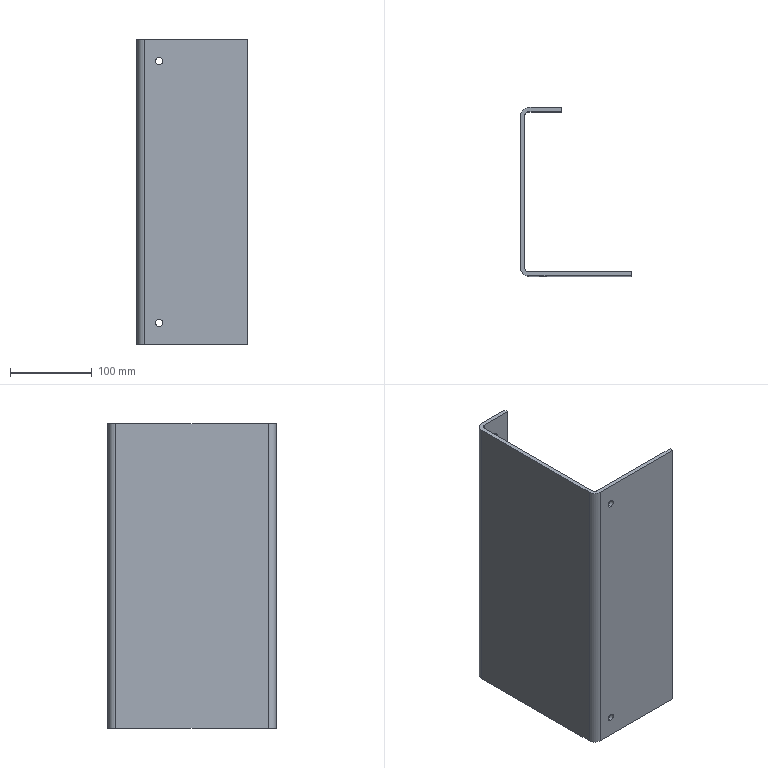Part | SolidWorks | features ExtruThin 1, ICE 1, LPattern 1 | 1 solid | 22 faces | box 135 x 206 x 372 mm | volume 695413 mm3 | cylinder 12 | plane 10 | commonest cylinder face diameters 9 x8 10 x2 20 x2
STEP:
#1=CARTESIAN_POINT('',(27.5,201.,21.5));
#2=VERTEX_POINT('',#1);
#3=CARTESIAN_POINT('',(27.5,201.,30.5));
#4=VERTEX_POINT('',#3);
#5=CARTESIAN_POINT('',(27.5,201.,26.));
#6=DIRECTION('',(0.,1.,0.));
#7=DIRECTION('',(0.,0.,1.));
#8=AXIS2_PLACEMENT_3D('',#5,#6,#7);
#9=CIRCLE('',#8,4.5);
#10=EDGE_CURVE('',#2,#4,#9,.T.);
#11=ORIENTED_EDGE('',*,*,#10,.F.);
#12=CARTESIAN_POINT('',(27.5,206.,21.5));
#13=VERTEX_POINT('',#12);
#14=CARTESIAN_POINT('',(27.5,0.,21.5));
#15=DIRECTION('',(0.,1.,0.));
#16=VECTOR('',#15,1000.);
#17=LINE('',#14,#16);
#18=EDGE_CURVE('',#2,#13,#17,.T.);
#19=ORIENTED_EDGE('',*,*,#18,.T.);
#20=CARTESIAN_POINT('',(27.5,206.,30.5));
#21=VERTEX_POINT('',#20);
#22=CARTESIAN_POINT('',(27.5,206.,26.));
#23=DIRECTION('',(0.,1.,0.));
#24=DIRECTION('',(0.,0.,1.));
#25=AXIS2_PLACEMENT_3D('',#22,#23,#24);
#26=CIRCLE('',#25,4.5);
#27=EDGE_CURVE('',#13,#21,#26,.T.);
#28=ORIENTED_EDGE('',*,*,#27,.T.);
#29=CARTESIAN_POINT('',(27.5,0.,30.5));
#30=DIRECTION('',(0.,1.,0.));
#31=VECTOR('',#30,1000.);
#32=LINE('',#29,#31);
#33=EDGE_CURVE('',#4,#21,#32,.T.);
#34=ORIENTED_EDGE('',*,*,#33,.F.);
#35=EDGE_LOOP('',(#11,#19,#28,#34));
#36=FACE_OUTER_BOUND('',#35,.T.);
#37=CARTESIAN_POINT('',(27.5,0.,26.));
#38=DIRECTION('',(0.,1.,0.));
#39=DIRECTION('',(0.,0.,1.));
#40=AXIS2_PLACEMENT_3D('',#37,#38,#39);
#41=CYLINDRICAL_SURFACE('',#40,4.5);
#42=ADVANCED_FACE('',(#36),#41,.F.);
#43=CARTESIAN_POINT('',(27.5,0.,21.5));
#44=VERTEX_POINT('',#43);
#45=CARTESIAN_POINT('',(27.5,0.,30.5));
#46=VERTEX_POINT('',#45);
#47=CARTESIAN_POINT('',(27.5,0.,26.));
#48=DIRECTION('',(0.,1.,0.));
#49=DIRECTION('',(0.,0.,1.));
#50=AXIS2_PLACEMENT_3D('',#47,#48,#49);
#51=CIRCLE('',#50,4.5);
#52=EDGE_CURVE('',#44,#46,#51,.T.);
#53=ORIENTED_EDGE('',*,*,#52,.F.);
#54=CARTESIAN_POINT('',(27.5,5.,21.5));
#55=VERTEX_POINT('',#54);
#56=CARTESIAN_POINT('',(27.5,0.,21.5));
#57=DIRECTION('',(0.,1.,0.));
#58=VECTOR('',#57,1000.);
#59=LINE('',#56,#58);
#60=EDGE_CURVE('',#44,#55,#59,.T.);
#61=ORIENTED_EDGE('',*,*,#60,.T.);
#62=CARTESIAN_POINT('',(27.5,5.,30.5));
#63=VERTEX_POINT('',#62);
#64=CARTESIAN_POINT('',(27.5,5.,26.));
#65=DIRECTION('',(0.,-1.,0.));
#66=DIRECTION('',(0.,0.,-1.));
#67=AXIS2_PLACEMENT_3D('',#64,#65,#66);
#68=CIRCLE('',#67,4.5);
#69=EDGE_CURVE('',#63,#55,#68,.T.);
#70=ORIENTED_EDGE('',*,*,#69,.F.);
#71=CARTESIAN_POINT('',(27.5,0.,30.5));
#72=DIRECTION('',(0.,1.,0.));
#73=VECTOR('',#72,1000.);
#74=LINE('',#71,#73);
#75=EDGE_CURVE('',#46,#63,#74,.T.);
#76=ORIENTED_EDGE('',*,*,#75,.F.);
#77=EDGE_LOOP('',(#53,#61,#70,#76));
#78=FACE_OUTER_BOUND('',#77,.T.);
#79=CARTESIAN_POINT('',(27.5,0.,26.));
#80=DIRECTION('',(0.,1.,0.));
#81=DIRECTION('',(0.,0.,1.));
#82=AXIS2_PLACEMENT_3D('',#79,#80,#81);
#83=CYLINDRICAL_SURFACE('',#82,4.5);
#84=ADVANCED_FACE('',(#78),#83,.F.);
#85=CARTESIAN_POINT('',(27.5,201.,341.5));
#86=VERTEX_POINT('',#85);
#87=CARTESIAN_POINT('',(27.5,201.,350.5));
#88=VERTEX_POINT('',#87);
#89=CARTESIAN_POINT('',(27.5,201.,346.));
#90=DIRECTION('',(0.,1.,0.));
#91=DIRECTION('',(0.,0.,1.));
#92=AXIS2_PLACEMENT_3D('',#89,#90,#91);
#93=CIRCLE('',#92,4.5);
#94=EDGE_CURVE('',#86,#88,#93,.T.);
#95=ORIENTED_EDGE('',*,*,#94,.F.);
#96=CARTESIAN_POINT('',(27.5,206.,341.5));
#97=VERTEX_POINT('',#96);
#98=CARTESIAN_POINT('',(27.5,0.,341.5));
#99=DIRECTION('',(0.,1.,0.));
#100=VECTOR('',#99,1000.);
#101=LINE('',#98,#100);
#102=EDGE_CURVE('',#86,#97,#101,.T.);
#103=ORIENTED_EDGE('',*,*,#102,.T.);
#104=CARTESIAN_POINT('',(27.5,206.,350.5));
#105=VERTEX_POINT('',#104);
#106=CARTESIAN_POINT('',(27.5,206.,346.));
#107=DIRECTION('',(0.,1.,0.));
#108=DIRECTION('',(0.,0.,1.));
#109=AXIS2_PLACEMENT_3D('',#106,#107,#108);
#110=CIRCLE('',#109,4.5);
#111=EDGE_CURVE('',#97,#105,#110,.T.);
#112=ORIENTED_EDGE('',*,*,#111,.T.);
#113=CARTESIAN_POINT('',(27.5,0.,350.5));
#114=DIRECTION('',(0.,1.,0.));
#115=VECTOR('',#114,1000.);
#116=LINE('',#113,#115);
#117=EDGE_CURVE('',#88,#105,#116,.T.);
#118=ORIENTED_EDGE('',*,*,#117,.F.);
#119=EDGE_LOOP('',(#95,#103,#112,#118));
#120=FACE_OUTER_BOUND('',#119,.T.);
#121=CARTESIAN_POINT('',(27.5,0.,346.));
#122=DIRECTION('',(0.,1.,0.));
#123=DIRECTION('',(0.,0.,1.));
#124=AXIS2_PLACEMENT_3D('',#121,#122,#123);
#125=CYLINDRICAL_SURFACE('',#124,4.5);
#126=ADVANCED_FACE('',(#120),#125,.F.);
#127=CARTESIAN_POINT('',(27.5,0.,341.5));
#128=VERTEX_POINT('',#127);
#129=CARTESIAN_POINT('',(27.5,0.,350.5));
#130=VERTEX_POINT('',#129);
#131=CARTESIAN_POINT('',(27.5,0.,346.));
#132=DIRECTION('',(0.,1.,0.));
#133=DIRECTION('',(0.,0.,1.));
#134=AXIS2_PLACEMENT_3D('',#131,#132,#133);
#135=CIRCLE('',#134,4.5);
#136=EDGE_CURVE('',#128,#130,#135,.T.);
#137=ORIENTED_EDGE('',*,*,#136,.F.);
#138=CARTESIAN_POINT('',(27.5,5.,341.5));
#139=VERTEX_POINT('',#138);
#140=CARTESIAN_POINT('',(27.5,0.,341.5));
#141=DIRECTION('',(0.,1.,0.));
#142=VECTOR('',#141,1000.);
#143=LINE('',#140,#142);
#144=EDGE_CURVE('',#128,#139,#143,.T.);
#145=ORIENTED_EDGE('',*,*,#144,.T.);
#146=CARTESIAN_POINT('',(27.5,5.,350.5));
#147=VERTEX_POINT('',#146);
#148=CARTESIAN_POINT('',(27.5,5.,346.));
#149=DIRECTION('',(0.,-1.,0.));
#150=DIRECTION('',(0.,0.,-1.));
#151=AXIS2_PLACEMENT_3D('',#148,#149,#150);
#152=CIRCLE('',#151,4.5);
#153=EDGE_CURVE('',#147,#139,#152,.T.);
#154=ORIENTED_EDGE('',*,*,#153,.F.);
#155=CARTESIAN_POINT('',(27.5,0.,350.5));
#156=DIRECTION('',(0.,1.,0.));
#157=VECTOR('',#156,1000.);
#158=LINE('',#155,#157);
#159=EDGE_CURVE('',#130,#147,#158,.T.);
#160=ORIENTED_EDGE('',*,*,#159,.F.);
#161=EDGE_LOOP('',(#137,#145,#154,#160));
#162=FACE_OUTER_BOUND('',#161,.T.);
#163=CARTESIAN_POINT('',(27.5,0.,346.));
#164=DIRECTION('',(0.,1.,0.));
#165=DIRECTION('',(0.,0.,1.));
#166=AXIS2_PLACEMENT_3D('',#163,#164,#165);
#167=CYLINDRICAL_SURFACE('',#166,4.5);
#168=ADVANCED_FACE('',(#162),#167,.F.);
#169=CARTESIAN_POINT('',(27.5,201.,26.));
#170=DIRECTION('',(0.,1.,0.));
#171=DIRECTION('',(0.,0.,1.));
#172=AXIS2_PLACEMENT_3D('',#169,#170,#171);
#173=CIRCLE('',#172,4.5);
#174=EDGE_CURVE('',#4,#2,#173,.T.);
#175=ORIENTED_EDGE('',*,*,#174,.T.);
#176=ORIENTED_EDGE('',*,*,#10,.T.);
#177=EDGE_LOOP('',(#175,#176));
#178=FACE_BOUND('',#177,.T.);
#179=CARTESIAN_POINT('',(27.5,201.,346.));
#180=DIRECTION('',(0.,1.,0.));
#181=DIRECTION('',(0.,0.,1.));
#182=AXIS2_PLACEMENT_3D('',#179,#180,#181);
#183=CIRCLE('',#182,4.5);
#184=EDGE_CURVE('',#88,#86,#183,.T.);
#185=ORIENTED_EDGE('',*,*,#184,.T.);
#186=ORIENTED_EDGE('',*,*,#94,.T.);
#187=EDGE_LOOP('',(#185,#186));
#188=FACE_BOUND('',#187,.T.);
#189=CARTESIAN_POINT('',(10.,201.,0.));
#190=VERTEX_POINT('',#189);
#191=CARTESIAN_POINT('',(50.,201.,0.));
#192=VERTEX_POINT('',#191);
#193=CARTESIAN_POINT('',(10.,201.,0.));
#194=DIRECTION('',(1.,0.,0.));
#195=VECTOR('',#194,1000.);
#196=LINE('',#193,#195);
#197=EDGE_CURVE('',#190,#192,#196,.T.);
#198=ORIENTED_EDGE('',*,*,#197,.T.);
#199=CARTESIAN_POINT('',(50.,201.,372.));
#200=VERTEX_POINT('',#199);
#201=CARTESIAN_POINT('',(50.,201.,372.));
#202=DIRECTION('',(0.,0.,-1.));
#203=VECTOR('',#202,1000.);
#204=LINE('',#201,#203);
#205=EDGE_CURVE('',#200,#192,#204,.T.);
#206=ORIENTED_EDGE('',*,*,#205,.F.);
#207=CARTESIAN_POINT('',(10.,201.,372.));
#208=VERTEX_POINT('',#207);
#209=CARTESIAN_POINT('',(10.,201.,372.));
#210=DIRECTION('',(1.,0.,0.));
#211=VECTOR('',#210,1000.);
#212=LINE('',#209,#211);
#213=EDGE_CURVE('',#208,#200,#212,.T.);
#214=ORIENTED_EDGE('',*,*,#213,.F.);
#215=CARTESIAN_POINT('',(10.,201.,372.));
#216=DIRECTION('',(0.,0.,-1.));
#217=VECTOR('',#216,1000.);
#218=LINE('',#215,#217);
#219=EDGE_CURVE('',#208,#190,#218,.T.);
#220=ORIENTED_EDGE('',*,*,#219,.T.);
#221=EDGE_LOOP('',(#198,#206,#214,#220));
#222=FACE_OUTER_BOUND('',#221,.T.);
#223=CARTESIAN_POINT('',(10.,201.,372.));
#224=DIRECTION('',(0.,1.,0.));
#225=DIRECTION('',(0.,0.,1.));
#226=AXIS2_PLACEMENT_3D('',#223,#224,#225);
#227=PLANE('',#226);
#228=ADVANCED_FACE('',(#178,#188,#222),#227,.F.);
#229=CARTESIAN_POINT('',(50.,206.,0.));
#230=VERTEX_POINT('',#229);
#231=CARTESIAN_POINT('',(50.,206.,0.));
#232=DIRECTION('',(0.,-1.,0.));
#233=VECTOR('',#232,1000.);
#234=LINE('',#231,#233);
#235=EDGE_CURVE('',#230,#192,#234,.T.);
#236=ORIENTED_EDGE('',*,*,#235,.F.);
#237=CARTESIAN_POINT('',(50.,206.,372.));
#238=VERTEX_POINT('',#237);
#239=CARTESIAN_POINT('',(50.,206.,372.));
#240=DIRECTION('',(0.,0.,-1.));
#241=VECTOR('',#240,1000.);
#242=LINE('',#239,#241);
#243=EDGE_CURVE('',#238,#230,#242,.T.);
#244=ORIENTED_EDGE('',*,*,#243,.F.);
#245=CARTESIAN_POINT('',(50.,206.,372.));
#246=DIRECTION('',(0.,-1.,0.));
#247=VECTOR('',#246,1000.);
#248=LINE('',#245,#247);
#249=EDGE_CURVE('',#238,#200,#248,.T.);
#250=ORIENTED_EDGE('',*,*,#249,.T.);
#251=ORIENTED_EDGE('',*,*,#205,.T.);
#252=EDGE_LOOP('',(#236,#244,#250,#251));
#253=FACE_OUTER_BOUND('',#252,.T.);
#254=CARTESIAN_POINT('',(50.,206.,372.));
#255=DIRECTION('',(1.,0.,0.));
#256=DIRECTION('',(0.,0.,-1.));
#257=AXIS2_PLACEMENT_3D('',#254,#255,#256);
#258=PLANE('',#257);
#259=ADVANCED_FACE('',(#253),#258,.T.);
#260=CARTESIAN_POINT('',(27.5,206.,26.));
#261=DIRECTION('',(0.,1.,0.));
#262=DIRECTION('',(0.,0.,1.));
#263=AXIS2_PLACEMENT_3D('',#260,#261,#262);
#264=CIRCLE('',#263,4.5);
#265=EDGE_CURVE('',#21,#13,#264,.T.);
#266=ORIENTED_EDGE('',*,*,#265,.F.);
#267=ORIENTED_EDGE('',*,*,#27,.F.);
#268=EDGE_LOOP('',(#266,#267));
#269=FACE_BOUND('',#268,.T.);
#270=CARTESIAN_POINT('',(27.5,206.,346.));
#271=DIRECTION('',(0.,1.,0.));
#272=DIRECTION('',(0.,0.,1.));
#273=AXIS2_PLACEMENT_3D('',#270,#271,#272);
#274=CIRCLE('',#273,4.5);
#275=EDGE_CURVE('',#105,#97,#274,.T.);
#276=ORIENTED_EDGE('',*,*,#275,.F.);
#277=ORIENTED_EDGE('',*,*,#111,.F.);
#278=EDGE_LOOP('',(#276,#277));
#279=FACE_BOUND('',#278,.T.);
#280=CARTESIAN_POINT('',(10.,206.,0.));
#281=VERTEX_POINT('',#280);
#282=CARTESIAN_POINT('',(10.,206.,0.));
#283=DIRECTION('',(1.,0.,0.));
#284=VECTOR('',#283,1000.);
#285=LINE('',#282,#284);
#286=EDGE_CURVE('',#281,#230,#285,.T.);
#287=ORIENTED_EDGE('',*,*,#286,.F.);
#288=CARTESIAN_POINT('',(10.,206.,372.));
#289=VERTEX_POINT('',#288);
#290=CARTESIAN_POINT('',(10.,206.,372.));
#291=DIRECTION('',(0.,0.,-1.));
#292=VECTOR('',#291,1000.);
#293=LINE('',#290,#292);
#294=EDGE_CURVE('',#289,#281,#293,.T.);
#295=ORIENTED_EDGE('',*,*,#294,.F.);
#296=CARTESIAN_POINT('',(10.,206.,372.));
#297=DIRECTION('',(1.,0.,0.));
#298=VECTOR('',#297,1000.);
#299=LINE('',#296,#298);
#300=EDGE_CURVE('',#289,#238,#299,.T.);
#301=ORIENTED_EDGE('',*,*,#300,.T.);
#302=ORIENTED_EDGE('',*,*,#243,.T.);
#303=EDGE_LOOP('',(#287,#295,#301,#302));
#304=FACE_OUTER_BOUND('',#303,.T.);
#305=CARTESIAN_POINT('',(10.,206.,372.));
#306=DIRECTION('',(0.,1.,0.));
#307=DIRECTION('',(0.,0.,1.));
#308=AXIS2_PLACEMENT_3D('',#305,#306,#307);
#309=PLANE('',#308);
#310=ADVANCED_FACE('',(#269,#279,#304),#309,.T.);
#311=CARTESIAN_POINT('',(0.,196.,0.));
#312=VERTEX_POINT('',#311);
#313=CARTESIAN_POINT('',(10.,196.,0.));
#314=DIRECTION('',(0.,0.,-1.));
#315=DIRECTION('',(1.,0.,0.));
#316=AXIS2_PLACEMENT_3D('',#313,#314,#315);
#317=CIRCLE('',#316,10.);
#318=EDGE_CURVE('',#312,#281,#317,.T.);
#319=ORIENTED_EDGE('',*,*,#318,.F.);
#320=CARTESIAN_POINT('',(0.,196.,372.));
#321=VERTEX_POINT('',#320);
#322=CARTESIAN_POINT('',(0.,196.,372.));
#323=DIRECTION('',(0.,0.,-1.));
#324=VECTOR('',#323,1000.);
#325=LINE('',#322,#324);
#326=EDGE_CURVE('',#321,#312,#325,.T.);
#327=ORIENTED_EDGE('',*,*,#326,.F.);
#328=CARTESIAN_POINT('',(10.,196.,372.));
#329=DIRECTION('',(0.,0.,-1.));
#330=DIRECTION('',(1.,0.,0.));
#331=AXIS2_PLACEMENT_3D('',#328,#329,#330);
#332=CIRCLE('',#331,10.);
#333=EDGE_CURVE('',#321,#289,#332,.T.);
#334=ORIENTED_EDGE('',*,*,#333,.T.);
#335=ORIENTED_EDGE('',*,*,#294,.T.);
#336=EDGE_LOOP('',(#319,#327,#334,#335));
#337=FACE_OUTER_BOUND('',#336,.T.);
#338=CARTESIAN_POINT('',(10.,196.,372.));
#339=DIRECTION('',(0.,0.,-1.));
#340=DIRECTION('',(-1.,0.,0.));
#341=AXIS2_PLACEMENT_3D('',#338,#339,#340);
#342=CYLINDRICAL_SURFACE('',#341,10.);
#343=ADVANCED_FACE('',(#337),#342,.T.);
#344=CARTESIAN_POINT('',(0.,10.,0.));
#345=VERTEX_POINT('',#344);
#346=CARTESIAN_POINT('',(0.,10.,0.));
#347=DIRECTION('',(0.,1.,0.));
#348=VECTOR('',#347,1000.);
#349=LINE('',#346,#348);
#350=EDGE_CURVE('',#345,#312,#349,.T.);
#351=ORIENTED_EDGE('',*,*,#350,.F.);
#352=CARTESIAN_POINT('',(0.,10.,372.));
#353=VERTEX_POINT('',#352);
#354=CARTESIAN_POINT('',(0.,10.,372.));
#355=DIRECTION('',(0.,0.,-1.));
#356=VECTOR('',#355,1000.);
#357=LINE('',#354,#356);
#358=EDGE_CURVE('',#353,#345,#357,.T.);
#359=ORIENTED_EDGE('',*,*,#358,.F.);
#360=CARTESIAN_POINT('',(0.,10.,372.));
#361=DIRECTION('',(0.,1.,0.));
#362=VECTOR('',#361,1000.);
#363=LINE('',#360,#362);
#364=EDGE_CURVE('',#353,#321,#363,.T.);
#365=ORIENTED_EDGE('',*,*,#364,.T.);
#366=ORIENTED_EDGE('',*,*,#326,.T.);
#367=EDGE_LOOP('',(#351,#359,#365,#366));
#368=FACE_OUTER_BOUND('',#367,.T.);
#369=CARTESIAN_POINT('',(0.,10.,372.));
#370=DIRECTION('',(-1.,0.,0.));
#371=DIRECTION('',(0.,0.,1.));
#372=AXIS2_PLACEMENT_3D('',#369,#370,#371);
#373=PLANE('',#372);
#374=ADVANCED_FACE('',(#368),#373,.T.);
#375=CARTESIAN_POINT('',(10.,0.,0.));
#376=VERTEX_POINT('',#375);
#377=CARTESIAN_POINT('',(10.,10.,0.));
#378=DIRECTION('',(0.,0.,-1.));
#379=DIRECTION('',(-1.,0.,0.));
#380=AXIS2_PLACEMENT_3D('',#377,#378,#379);
#381=CIRCLE('',#380,10.);
#382=EDGE_CURVE('',#376,#345,#381,.T.);
#383=ORIENTED_EDGE('',*,*,#382,.F.);
#384=CARTESIAN_POINT('',(10.,0.,372.));
#385=VERTEX_POINT('',#384);
#386=CARTESIAN_POINT('',(10.,0.,372.));
#387=DIRECTION('',(0.,0.,-1.));
#388=VECTOR('',#387,1000.);
#389=LINE('',#386,#388);
#390=EDGE_CURVE('',#385,#376,#389,.T.);
#391=ORIENTED_EDGE('',*,*,#390,.F.);
#392=CARTESIAN_POINT('',(10.,10.,372.));
#393=DIRECTION('',(0.,0.,-1.));
#394=DIRECTION('',(-1.,0.,0.));
#395=AXIS2_PLACEMENT_3D('',#392,#393,#394);
#396=CIRCLE('',#395,10.);
#397=EDGE_CURVE('',#385,#353,#396,.T.);
#398=ORIENTED_EDGE('',*,*,#397,.T.);
#399=ORIENTED_EDGE('',*,*,#358,.T.);
#400=EDGE_LOOP('',(#383,#391,#398,#399));
#401=FACE_OUTER_BOUND('',#400,.T.);
#402=CARTESIAN_POINT('',(10.,10.,372.));
#403=DIRECTION('',(0.,0.,-1.));
#404=DIRECTION('',(-1.,0.,0.));
#405=AXIS2_PLACEMENT_3D('',#402,#403,#404);
#406=CYLINDRICAL_SURFACE('',#405,10.);
#407=ADVANCED_FACE('',(#401),#406,.T.);
#408=CARTESIAN_POINT('',(27.5,0.,26.));
#409=DIRECTION('',(0.,1.,0.));
#410=DIRECTION('',(0.,0.,1.));
#411=AXIS2_PLACEMENT_3D('',#408,#409,#410);
#412=CIRCLE('',#411,4.5);
#413=EDGE_CURVE('',#46,#44,#412,.T.);
#414=ORIENTED_EDGE('',*,*,#413,.T.);
#415=ORIENTED_EDGE('',*,*,#52,.T.);
#416=EDGE_LOOP('',(#414,#415));
#417=FACE_BOUND('',#416,.T.);
#418=CARTESIAN_POINT('',(27.5,0.,346.));
#419=DIRECTION('',(0.,1.,0.));
#420=DIRECTION('',(0.,0.,1.));
#421=AXIS2_PLACEMENT_3D('',#418,#419,#420);
#422=CIRCLE('',#421,4.5);
#423=EDGE_CURVE('',#130,#128,#422,.T.);
#424=ORIENTED_EDGE('',*,*,#423,.T.);
#425=ORIENTED_EDGE('',*,*,#136,.T.);
#426=EDGE_LOOP('',(#424,#425));
#427=FACE_BOUND('',#426,.T.);
#428=CARTESIAN_POINT('',(135.,0.,0.));
#429=VERTEX_POINT('',#428);
#430=CARTESIAN_POINT('',(10.,0.,0.));
#431=DIRECTION('',(-1.,0.,0.));
#432=VECTOR('',#431,1000.);
#433=LINE('',#430,#432);
#434=EDGE_CURVE('',#429,#376,#433,.T.);
#435=ORIENTED_EDGE('',*,*,#434,.F.);
#436=CARTESIAN_POINT('',(135.,0.,372.));
#437=VERTEX_POINT('',#436);
#438=CARTESIAN_POINT('',(135.,0.,372.));
#439=DIRECTION('',(0.,0.,-1.));
#440=VECTOR('',#439,1000.);
#441=LINE('',#438,#440);
#442=EDGE_CURVE('',#437,#429,#441,.T.);
#443=ORIENTED_EDGE('',*,*,#442,.F.);
#444=CARTESIAN_POINT('',(10.,0.,372.));
#445=DIRECTION('',(-1.,0.,0.));
#446=VECTOR('',#445,1000.);
#447=LINE('',#444,#446);
#448=EDGE_CURVE('',#437,#385,#447,.T.);
#449=ORIENTED_EDGE('',*,*,#448,.T.);
#450=ORIENTED_EDGE('',*,*,#390,.T.);
#451=EDGE_LOOP('',(#435,#443,#449,#450));
#452=FACE_OUTER_BOUND('',#451,.T.);
#453=CARTESIAN_POINT('',(10.,0.,372.));
#454=DIRECTION('',(0.,-1.,0.));
#455=DIRECTION('',(0.,0.,-1.));
#456=AXIS2_PLACEMENT_3D('',#453,#454,#455);
#457=PLANE('',#456);
#458=ADVANCED_FACE('',(#417,#427,#452),#457,.T.);
#459=CARTESIAN_POINT('',(135.,5.,0.));
#460=VERTEX_POINT('',#459);
#461=CARTESIAN_POINT('',(135.,5.,0.));
#462=DIRECTION('',(0.,-1.,0.));
#463=VECTOR('',#462,1000.);
#464=LINE('',#461,#463);
#465=EDGE_CURVE('',#460,#429,#464,.T.);
#466=ORIENTED_EDGE('',*,*,#465,.F.);
#467=CARTESIAN_POINT('',(135.,5.,372.));
#468=VERTEX_POINT('',#467);
#469=CARTESIAN_POINT('',(135.,5.,372.));
#470=DIRECTION('',(0.,0.,-1.));
#471=VECTOR('',#470,1000.);
#472=LINE('',#469,#471);
#473=EDGE_CURVE('',#468,#460,#472,.T.);
#474=ORIENTED_EDGE('',*,*,#473,.F.);
#475=CARTESIAN_POINT('',(135.,5.,372.));
#476=DIRECTION('',(0.,-1.,0.));
#477=VECTOR('',#476,1000.);
#478=LINE('',#475,#477);
#479=EDGE_CURVE('',#468,#437,#478,.T.);
#480=ORIENTED_EDGE('',*,*,#479,.T.);
#481=ORIENTED_EDGE('',*,*,#442,.T.);
#482=EDGE_LOOP('',(#466,#474,#480,#481));
#483=FACE_OUTER_BOUND('',#482,.T.);
#484=CARTESIAN_POINT('',(135.,5.,372.));
#485=DIRECTION('',(1.,0.,0.));
#486=DIRECTION('',(0.,0.,-1.));
#487=AXIS2_PLACEMENT_3D('',#484,#485,#486);
#488=PLANE('',#487);
#489=ADVANCED_FACE('',(#483),#488,.T.);
#490=ORIENTED_EDGE('',*,*,#69,.T.);
#491=CARTESIAN_POINT('',(27.5,5.,26.));
#492=DIRECTION('',(0.,-1.,0.));
#493=DIRECTION('',(0.,0.,-1.));
#494=AXIS2_PLACEMENT_3D('',#491,#492,#493);
#495=CIRCLE('',#494,4.5);
#496=EDGE_CURVE('',#55,#63,#495,.T.);
#497=ORIENTED_EDGE('',*,*,#496,.T.);
#498=EDGE_LOOP('',(#490,#497));
#499=FACE_BOUND('',#498,.T.);
#500=ORIENTED_EDGE('',*,*,#153,.T.);
#501=CARTESIAN_POINT('',(27.5,5.,346.));
#502=DIRECTION('',(0.,-1.,0.));
#503=DIRECTION('',(0.,0.,-1.));
#504=AXIS2_PLACEMENT_3D('',#501,#502,#503);
#505=CIRCLE('',#504,4.5);
#506=EDGE_CURVE('',#139,#147,#505,.T.);
#507=ORIENTED_EDGE('',*,*,#506,.T.);
#508=EDGE_LOOP('',(#500,#507));
#509=FACE_BOUND('',#508,.T.);
#510=CARTESIAN_POINT('',(10.,5.,0.));
#511=VERTEX_POINT('',#510);
#512=CARTESIAN_POINT('',(10.,5.,0.));
#513=DIRECTION('',(-1.,0.,0.));
#514=VECTOR('',#513,1000.);
#515=LINE('',#512,#514);
#516=EDGE_CURVE('',#460,#511,#515,.T.);
#517=ORIENTED_EDGE('',*,*,#516,.T.);
#518=CARTESIAN_POINT('',(10.,5.,372.));
#519=VERTEX_POINT('',#518);
#520=CARTESIAN_POINT('',(10.,5.,372.));
#521=DIRECTION('',(0.,0.,-1.));
#522=VECTOR('',#521,1000.);
#523=LINE('',#520,#522);
#524=EDGE_CURVE('',#519,#511,#523,.T.);
#525=ORIENTED_EDGE('',*,*,#524,.F.);
#526=CARTESIAN_POINT('',(10.,5.,372.));
#527=DIRECTION('',(-1.,0.,0.));
#528=VECTOR('',#527,1000.);
#529=LINE('',#526,#528);
#530=EDGE_CURVE('',#468,#519,#529,.T.);
#531=ORIENTED_EDGE('',*,*,#530,.F.);
#532=ORIENTED_EDGE('',*,*,#473,.T.);
#533=EDGE_LOOP('',(#517,#525,#531,#532));
#534=FACE_OUTER_BOUND('',#533,.T.);
#535=CARTESIAN_POINT('',(10.,5.,372.));
#536=DIRECTION('',(0.,-1.,0.));
#537=DIRECTION('',(0.,0.,-1.));
#538=AXIS2_PLACEMENT_3D('',#535,#536,#537);
#539=PLANE('',#538);
#540=ADVANCED_FACE('',(#499,#509,#534),#539,.F.);
#541=CARTESIAN_POINT('',(5.,10.,0.));
#542=VERTEX_POINT('',#541);
#543=CARTESIAN_POINT('',(10.,10.,0.));
#544=DIRECTION('',(0.,0.,-1.));
#545=DIRECTION('',(1.,0.,0.));
#546=AXIS2_PLACEMENT_3D('',#543,#544,#545);
#547=CIRCLE('',#546,5.);
#548=EDGE_CURVE('',#511,#542,#547,.T.);
#549=ORIENTED_EDGE('',*,*,#548,.T.);
#550=CARTESIAN_POINT('',(5.,10.,372.));
#551=VERTEX_POINT('',#550);
#552=CARTESIAN_POINT('',(5.,10.,372.));
#553=DIRECTION('',(0.,0.,-1.));
#554=VECTOR('',#553,1000.);
#555=LINE('',#552,#554);
#556=EDGE_CURVE('',#551,#542,#555,.T.);
#557=ORIENTED_EDGE('',*,*,#556,.F.);
#558=CARTESIAN_POINT('',(10.,10.,372.));
#559=DIRECTION('',(0.,0.,-1.));
#560=DIRECTION('',(1.,0.,0.));
#561=AXIS2_PLACEMENT_3D('',#558,#559,#560);
#562=CIRCLE('',#561,5.);
#563=EDGE_CURVE('',#519,#551,#562,.T.);
#564=ORIENTED_EDGE('',*,*,#563,.F.);
#565=ORIENTED_EDGE('',*,*,#524,.T.);
#566=EDGE_LOOP('',(#549,#557,#564,#565));
#567=FACE_OUTER_BOUND('',#566,.T.);
#568=CARTESIAN_POINT('',(10.,10.,372.));
#569=DIRECTION('',(0.,0.,-1.));
#570=DIRECTION('',(-1.,0.,0.));
#571=AXIS2_PLACEMENT_3D('',#568,#569,#570);
#572=CYLINDRICAL_SURFACE('',#571,5.);
#573=ADVANCED_FACE('',(#567),#572,.F.);
#574=CARTESIAN_POINT('',(5.,196.,0.));
#575=VERTEX_POINT('',#574);
#576=CARTESIAN_POINT('',(5.,10.,0.));
#577=DIRECTION('',(0.,1.,0.));
#578=VECTOR('',#577,1000.);
#579=LINE('',#576,#578);
#580=EDGE_CURVE('',#542,#575,#579,.T.);
#581=ORIENTED_EDGE('',*,*,#580,.T.);
#582=CARTESIAN_POINT('',(5.,196.,372.));
#583=VERTEX_POINT('',#582);
#584=CARTESIAN_POINT('',(5.,196.,372.));
#585=DIRECTION('',(0.,0.,-1.));
#586=VECTOR('',#585,1000.);
#587=LINE('',#584,#586);
#588=EDGE_CURVE('',#583,#575,#587,.T.);
#589=ORIENTED_EDGE('',*,*,#588,.F.);
#590=CARTESIAN_POINT('',(5.,10.,372.));
#591=DIRECTION('',(0.,1.,0.));
#592=VECTOR('',#591,1000.);
#593=LINE('',#590,#592);
#594=EDGE_CURVE('',#551,#583,#593,.T.);
#595=ORIENTED_EDGE('',*,*,#594,.F.);
#596=ORIENTED_EDGE('',*,*,#556,.T.);
#597=EDGE_LOOP('',(#581,#589,#595,#596));
#598=FACE_OUTER_BOUND('',#597,.T.);
#599=CARTESIAN_POINT('',(5.,10.,372.));
#600=DIRECTION('',(-1.,0.,0.));
#601=DIRECTION('',(0.,0.,1.));
#602=AXIS2_PLACEMENT_3D('',#599,#600,#601);
#603=PLANE('',#602);
#604=ADVANCED_FACE('',(#598),#603,.F.);
#605=CARTESIAN_POINT('',(10.,196.,0.));
#606=DIRECTION('',(0.,0.,-1.));
#607=DIRECTION('',(1.,0.,0.));
#608=AXIS2_PLACEMENT_3D('',#605,#606,#607);
#609=CIRCLE('',#608,5.);
#610=EDGE_CURVE('',#575,#190,#609,.T.);
#611=ORIENTED_EDGE('',*,*,#610,.T.);
#612=ORIENTED_EDGE('',*,*,#219,.F.);
#613=CARTESIAN_POINT('',(10.,196.,372.));
#614=DIRECTION('',(0.,0.,-1.));
#615=DIRECTION('',(1.,0.,0.));
#616=AXIS2_PLACEMENT_3D('',#613,#614,#615);
#617=CIRCLE('',#616,5.);
#618=EDGE_CURVE('',#583,#208,#617,.T.);
#619=ORIENTED_EDGE('',*,*,#618,.F.);
#620=ORIENTED_EDGE('',*,*,#588,.T.);
#621=EDGE_LOOP('',(#611,#612,#619,#620));
#622=FACE_OUTER_BOUND('',#621,.T.);
#623=CARTESIAN_POINT('',(10.,196.,372.));
#624=DIRECTION('',(0.,0.,-1.));
#625=DIRECTION('',(-1.,0.,0.));
#626=AXIS2_PLACEMENT_3D('',#623,#624,#625);
#627=CYLINDRICAL_SURFACE('',#626,5.);
#628=ADVANCED_FACE('',(#622),#627,.F.);
#629=ORIENTED_EDGE('',*,*,#213,.T.);
#630=ORIENTED_EDGE('',*,*,#249,.F.);
#631=ORIENTED_EDGE('',*,*,#300,.F.);
#632=ORIENTED_EDGE('',*,*,#333,.F.);
#633=ORIENTED_EDGE('',*,*,#364,.F.);
#634=ORIENTED_EDGE('',*,*,#397,.F.);
#635=ORIENTED_EDGE('',*,*,#448,.F.);
#636=ORIENTED_EDGE('',*,*,#479,.F.);
#637=ORIENTED_EDGE('',*,*,#530,.T.);
#638=ORIENTED_EDGE('',*,*,#563,.T.);
#639=ORIENTED_EDGE('',*,*,#594,.T.);
#640=ORIENTED_EDGE('',*,*,#618,.T.);
#641=EDGE_LOOP('',(#629,#630,#631,#632,#633,#634,#635,#636,#637,#638,#639,#640));
#642=FACE_OUTER_BOUND('',#641,.T.);
#643=CARTESIAN_POINT('',(10.,196.,372.));
#644=DIRECTION('',(0.,0.,-1.));
#645=DIRECTION('',(-1.,0.,0.));
#646=AXIS2_PLACEMENT_3D('',#643,#644,#645);
#647=PLANE('',#646);
#648=ADVANCED_FACE('',(#642),#647,.F.);
#649=ORIENTED_EDGE('',*,*,#197,.F.);
#650=ORIENTED_EDGE('',*,*,#610,.F.);
#651=ORIENTED_EDGE('',*,*,#580,.F.);
#652=ORIENTED_EDGE('',*,*,#548,.F.);
#653=ORIENTED_EDGE('',*,*,#516,.F.);
#654=ORIENTED_EDGE('',*,*,#465,.T.);
#655=ORIENTED_EDGE('',*,*,#434,.T.);
#656=ORIENTED_EDGE('',*,*,#382,.T.);
#657=ORIENTED_EDGE('',*,*,#350,.T.);
#658=ORIENTED_EDGE('',*,*,#318,.T.);
#659=ORIENTED_EDGE('',*,*,#286,.T.);
#660=ORIENTED_EDGE('',*,*,#235,.T.);
#661=EDGE_LOOP('',(#649,#650,#651,#652,#653,#654,#655,#656,#657,#658,#659,#660));
#662=FACE_OUTER_BOUND('',#661,.T.);
#663=CARTESIAN_POINT('',(10.,196.,0.));
#664=DIRECTION('',(0.,0.,-1.));
#665=DIRECTION('',(-1.,0.,0.));
#666=AXIS2_PLACEMENT_3D('',#663,#664,#665);
#667=PLANE('',#666);
#668=ADVANCED_FACE('',(#662),#667,.T.);
#669=ORIENTED_EDGE('',*,*,#144,.F.);
#670=ORIENTED_EDGE('',*,*,#423,.F.);
#671=ORIENTED_EDGE('',*,*,#159,.T.);
#672=ORIENTED_EDGE('',*,*,#506,.F.);
#673=EDGE_LOOP('',(#669,#670,#671,#672));
#674=FACE_OUTER_BOUND('',#673,.T.);
#675=CARTESIAN_POINT('',(27.5,0.,346.));
#676=DIRECTION('',(0.,1.,0.));
#677=DIRECTION('',(0.,0.,1.));
#678=AXIS2_PLACEMENT_3D('',#675,#676,#677);
#679=CYLINDRICAL_SURFACE('',#678,4.5);
#680=ADVANCED_FACE('',(#674),#679,.F.);
#681=ORIENTED_EDGE('',*,*,#102,.F.);
#682=ORIENTED_EDGE('',*,*,#184,.F.);
#683=ORIENTED_EDGE('',*,*,#117,.T.);
#684=ORIENTED_EDGE('',*,*,#275,.T.);
#685=EDGE_LOOP('',(#681,#682,#683,#684));
#686=FACE_OUTER_BOUND('',#685,.T.);
#687=CARTESIAN_POINT('',(27.5,0.,346.));
#688=DIRECTION('',(0.,1.,0.));
#689=DIRECTION('',(0.,0.,1.));
#690=AXIS2_PLACEMENT_3D('',#687,#688,#689);
#691=CYLINDRICAL_SURFACE('',#690,4.5);
#692=ADVANCED_FACE('',(#686),#691,.F.);
#693=ORIENTED_EDGE('',*,*,#60,.F.);
#694=ORIENTED_EDGE('',*,*,#413,.F.);
#695=ORIENTED_EDGE('',*,*,#75,.T.);
#696=ORIENTED_EDGE('',*,*,#496,.F.);
#697=EDGE_LOOP('',(#693,#694,#695,#696));
#698=FACE_OUTER_BOUND('',#697,.T.);
#699=CARTESIAN_POINT('',(27.5,0.,26.));
#700=DIRECTION('',(0.,1.,0.));
#701=DIRECTION('',(0.,0.,1.));
#702=AXIS2_PLACEMENT_3D('',#699,#700,#701);
#703=CYLINDRICAL_SURFACE('',#702,4.5);
#704=ADVANCED_FACE('',(#698),#703,.F.);
#705=ORIENTED_EDGE('',*,*,#18,.F.);
#706=ORIENTED_EDGE('',*,*,#174,.F.);
#707=ORIENTED_EDGE('',*,*,#33,.T.);
#708=ORIENTED_EDGE('',*,*,#265,.T.);
#709=EDGE_LOOP('',(#705,#706,#707,#708));
#710=FACE_OUTER_BOUND('',#709,.T.);
#711=CARTESIAN_POINT('',(27.5,0.,26.));
#712=DIRECTION('',(0.,1.,0.));
#713=DIRECTION('',(0.,0.,1.));
#714=AXIS2_PLACEMENT_3D('',#711,#712,#713);
#715=CYLINDRICAL_SURFACE('',#714,4.5);
#716=ADVANCED_FACE('',(#710),#715,.F.);
#717=CLOSED_SHELL('',(#42,#84,#126,#168,#228,#259,#310,#343,#374,#407,#458,#489,#540,#573,#604,#628,#648,#668,#680,#692,#704,#716));
#718=MANIFOLD_SOLID_BREP('',#717);
#719=CARTESIAN_POINT('',(0.,0.,0.));
#720=DIRECTION('',(0.,0.,1.));
#721=DIRECTION('',(1.,0.,0.));
#722=AXIS2_PLACEMENT_3D('',#719,#720,#721);
#723=(LENGTH_UNIT()NAMED_UNIT(*)SI_UNIT(.MILLI.,.METRE.));
#724=UNCERTAINTY_MEASURE_WITH_UNIT(LENGTH_MEASURE(0.00001),#723,'','');
#725=(NAMED_UNIT(*)PLANE_ANGLE_UNIT()SI_UNIT($,.RADIAN.));
#726=(NAMED_UNIT(*)SI_UNIT($,.STERADIAN.)SOLID_ANGLE_UNIT());
#727=(GEOMETRIC_REPRESENTATION_CONTEXT(3)GLOBAL_UNCERTAINTY_ASSIGNED_CONTEXT((#724))GLOBAL_UNIT_ASSIGNED_CONTEXT((#723,#725,#726))REPRESENTATION_CONTEXT('',''));
#728=ADVANCED_BREP_SHAPE_REPRESENTATION('',(#718,#722),#727);